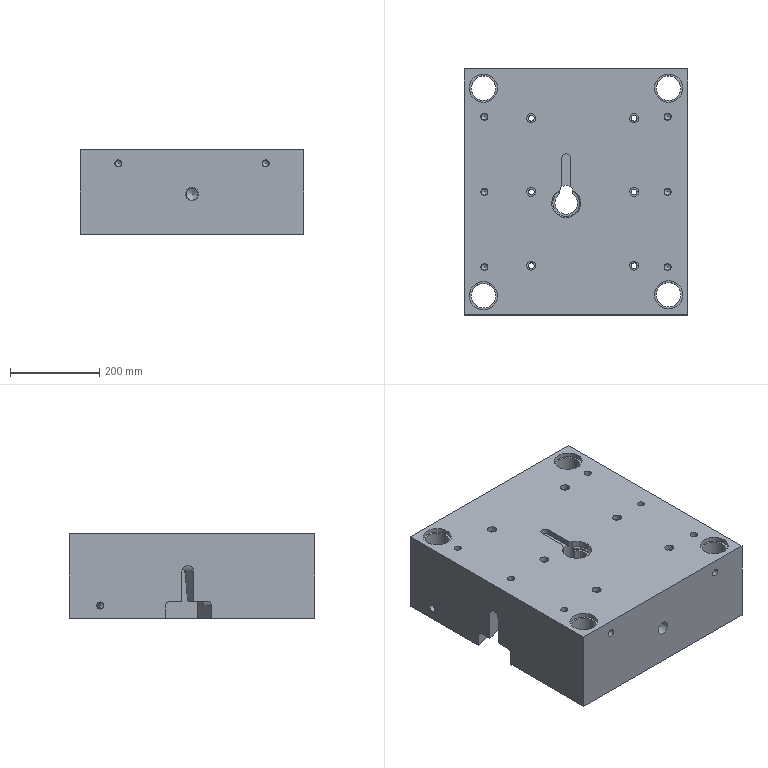Part | STEP file | 车灯-后视镜_id502_x_t | 1 solid | 254 faces | box 500 x 550 x 190 mm | volume 33080670 mm3 | cylinder 123 | plane 96 | cone 29 | sphere 4 | spline 2 | commonest cylinder face diameters 8 x20 20 x17 16 x14 5.1 x13 6 x13 13 x6